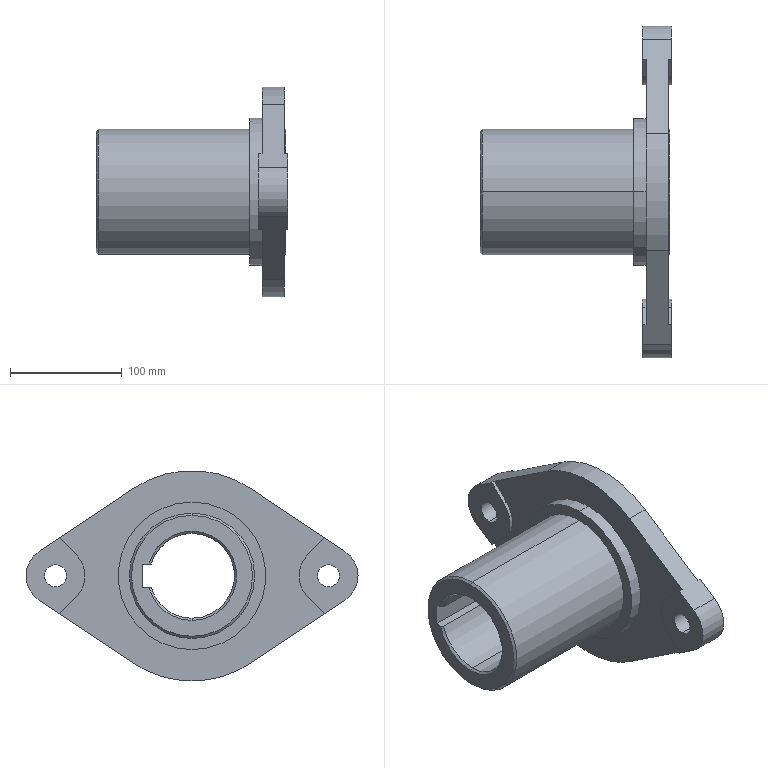Part | NX | features BREP 1, SCALE 1 | 1 solid | 51 faces | box 171.496 x 296.82 x 187.986 mm | volume 1461921 mm3 | plane 24 | cylinder 22 | cone 5 | commonest cylinder face diameters 52.768 x6 19.788 x4 112.132 x4 75.854 x3 187.986 x3 131.92 x2